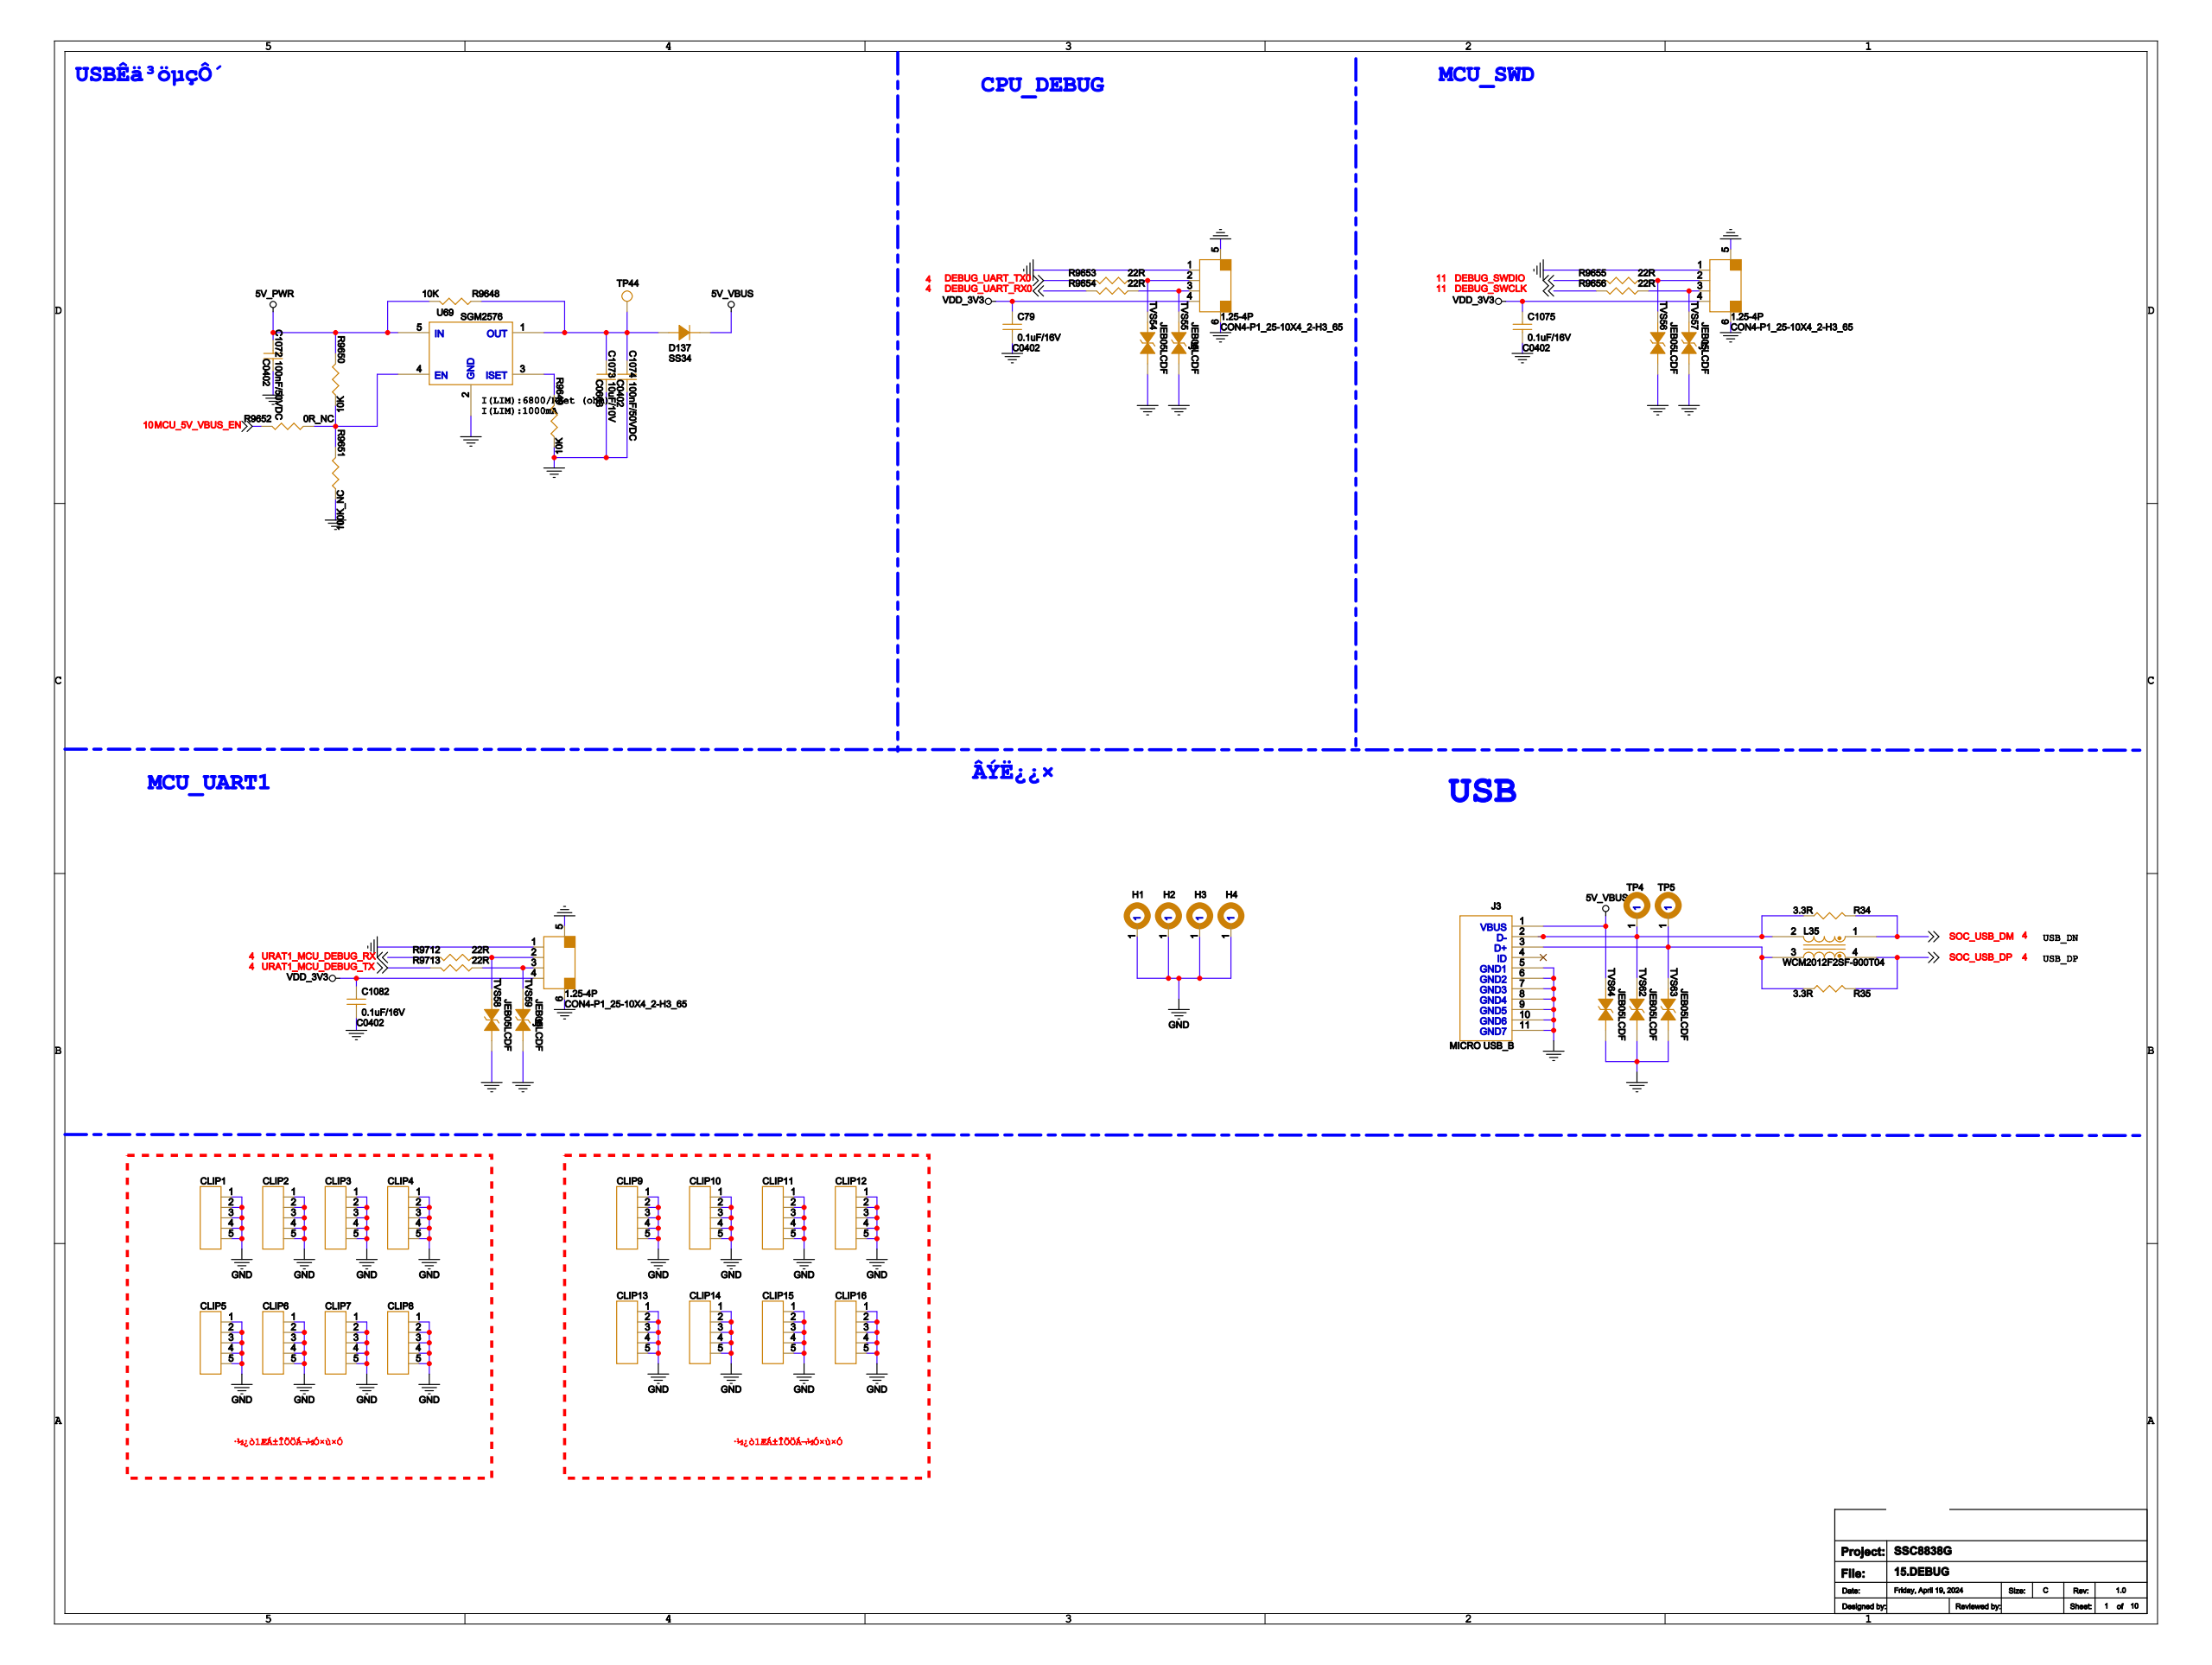Circuit board | Cadence Allegro | 958 parts | 601 nets | one sheet of the schematic
Parts on this sheet (reference | value | footprint):
C79 | 0.1uF/16V | C0402
C1072 | 100nF/50VDC | C0402
C1073 | 10uF/10V | C0603
C1074 | 100nF/50VDC | C0402
C1075 | 0.1uF/16V | C0402
C1082 | 0.1uF/16V | C0402
CLIP1 | DCL-PBJ001 | PBJ-01
CLIP2 | DCL-PBJ001 | PBJ-01
CLIP3 | DCL-PBJ001 | PBJ-01
CLIP4 | DCL-PBJ001 | PBJ-01
CLIP5 | DCL-PBJ001 | PBJ-01
CLIP6 | DCL-PBJ001 | PBJ-01
CLIP7 | DCL-PBJ001 | PBJ-01
CLIP8 | DCL-PBJ001 | PBJ-01
CLIP9 | DCL-PBJ001 | PBJ-01
CLIP10 | DCL-PBJ001 | PBJ-01
CLIP11 | DCL-PBJ001 | PBJ-01
CLIP12 | DCL-PBJ001 | PBJ-01
CLIP13 | DCL-PBJ001 | PBJ-01
CLIP14 | DCL-PBJ001 | PBJ-01
CLIP15 | DCL-PBJ001 | PBJ-01
CLIP16 | DCL-PBJ001 | PBJ-01
D137 | SS34 | SMB
J3 | MICRO USB_B | USB5_5X6_9H2_35_L1_6
J6 | 1.25-4P | CON4-P1_25-10X4_2-H3_65
J7 | 1.25-4P | CON4-P1_25-10X4_2-H3_65
J8 | 1.25-4P | CON4-P1_25-10X4_2-H3_65
L35 | WCM2012F2SF-900T04 | ESD4_0_9X0_7H0
R34 | 3.3R | R0402
R35 | 3.3R | R0402
R9648 | 10K | R0603
R9649 | 10K | R0402
R9650 | 10K | R0402
R9651 | 100K_NC | R0402
R9652 | 0R_NC | R0402
R9653 | 22R | R0402
R9654 | 22R | R0402
R9655 | 22R | R0402
R9656 | 22R | R0402
R9712 | 22R | R0402
R9713 | 22R | R0402
TP4 | HOLE | TP-C40
TP5 | HOLE | TP-C40
TP44 | Test_Point | TP_0R50
TVS54 | JEB05LCDF | R0402
TVS55 | JEB05LCDF | R0402
TVS56 | JEB05LCDF | TVS0402
TVS57 | JEB05LCDF | R0402
TVS58 | JEB05LCDF | R0402
TVS59 | JEB05LCDF | R0402
TVS62 | JEB05LCDF | TVS0402
TVS63 | JEB05LCDF | R0402
TVS64 | JEB05LCDF | R0402
U69 | SGM2576 | SOT23-5
Nets of these parts (net: part-pin ...):
GND: C79-2 C1072-1 C1073-1 C1074-1 C1075-2 C1082-2 CLIP1-1 CLIP1-2 CLIP1-3 CLIP1-4 CLIP1-5 CLIP2-1 CLIP2-2 CLIP2-3 CLIP2-4 CLIP2-5 CLIP3-1 CLIP3-2 CLIP3-3 CLIP3-4 CLIP3-5 CLIP4-1 CLIP4-2 CLIP4-3 CLIP4-4 CLIP4-5 CLIP5-1 CLIP5-2 CLIP5-3 CLIP5-4 CLIP5-5 CLIP6-1 CLIP6-2 CLIP6-3 CLIP6-4 CLIP6-5 CLIP7-1 CLIP7-2 CLIP7-3 CLIP7-4 CLIP7-5 CLIP8-1 CLIP8-2 CLIP8-3 CLIP8-4 CLIP8-5 CLIP9-1 CLIP9-2 CLIP9-3 CLIP9-4 CLIP9-5 CLIP10-1 CLIP10-2 CLIP10-3 CLIP10-4 CLIP10-5 CLIP11-1 CLIP11-2 CLIP11-3 CLIP11-4 CLIP11-5 CLIP12-1 CLIP12-2 CLIP12-3 CLIP12-4 CLIP12-5 CLIP13-1 CLIP13-2 CLIP13-3 CLIP13-4 CLIP13-5 CLIP14-1 CLIP14-2 CLIP14-3 CLIP14-4 CLIP14-5 CLIP15-1 CLIP15-2 CLIP15-3 CLIP15-4 CLIP15-5 CLIP16-1 CLIP16-2 CLIP16-3 CLIP16-4 CLIP16-5 J3-5 J3-6 J3-7 J3-8 J3-9 J3-10 J3-11 J6-1 J6-5 J6-6 J7-1 J7-5 J7-6 J8-1 J8-5 J8-6 R9649-2 R9651-2 TVS54-1 TVS55-1 TVS56-1 TVS57-1 TVS58-1 TVS59-1 TVS62-1 TVS63-1 TVS64-1 U69-2
5V_PWR: C1072-2 R9648-1 R9650-1 U69-5
3V3_NORMAL: C79-1 C1075-1 C1082-1 J6-4 J7-4 J8-4
N21292323: C1073-2 C1074-2 D137-1 R9648-2 TP44-1 U69-1
5V_VBUS: D137-2 J3-1 TVS64-2
N22032033: J3-3 L35-3 R35-2 TP5-1 TVS63-2
N22032114: J3-2 L35-2 R34-2 TP4-1 TVS62-2
N21294442: J6-2 R9653-2 TVS54-2
N21294472: J6-3 R9654-2 TVS55-2
N21295269: J7-2 R9655-2 TVS56-2
N21295279: J7-3 R9656-2 TVS57-2
N21371060: J8-2 R9712-2 TVS58-2
N21371062: J8-3 R9713-2 TVS59-2
SOC_USB_DM: L35-1 R34-1
SOC_USB_DP: L35-4 R35-1
DEBUG_SWDIO: R9655-1
N21292365: R9649-1 U69-3
N21292448: R9650-2 R9651-1 R9652-2 U69-4
DEBUG_UART_TX0: R9653-1
DEBUG_UART_RX0: R9654-1
DEBUG_SWCLK: R9656-1
URAT1_MCU_DEBUG_RX: R9712-1
URAT1_MCU_DEBUG_TX: R9713-1
MCU_5V_VBUS_EN: R9652-1